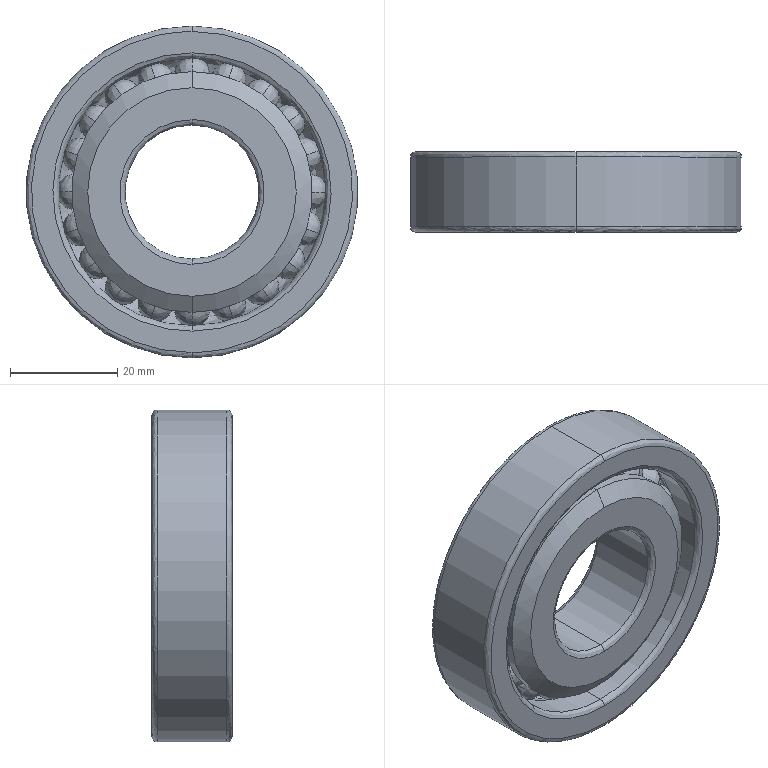Part | STEP file | 25TAC628B Bearing | 3 solids | 456 faces | box 62 x 15 x 62 mm | volume 31860 mm3 | plane 228 | spline 212 | cylinder 12 | cone 4 | commonest cylinder face diameters 25 x2 37 x2 42 x2 45 x2 50 x2 62 x2